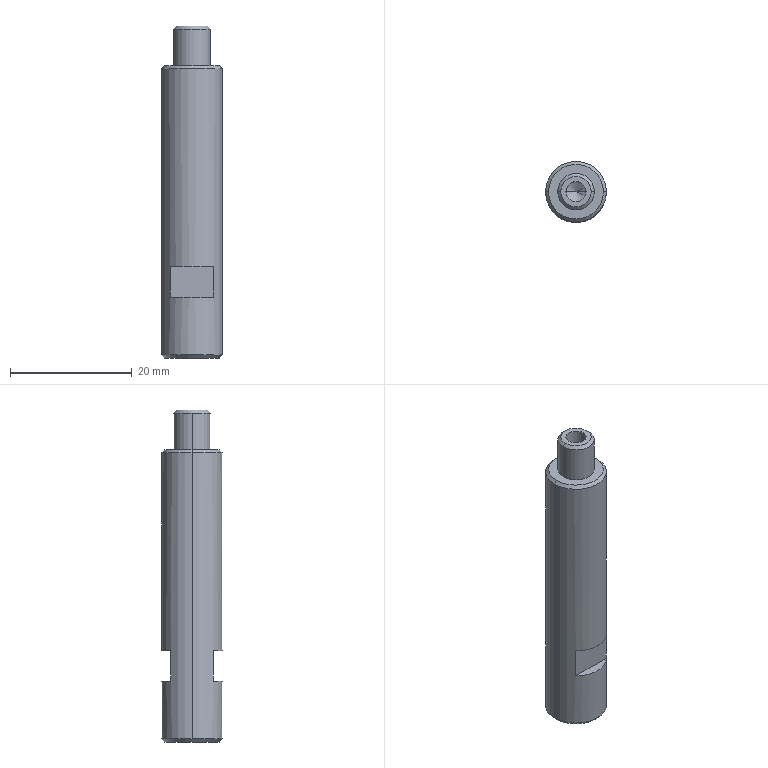Part | SolidWorks | features HoleWzd 2, ICE 2, Chamfer 1, Extrusion 1, MirrorPattern 1 | 1 solid | 27 faces | box 10 x 10 x 54.5 mm | volume 3603 mm3 | cone 10 | plane 9 | cylinder 8 | commonest cylinder face diameters 3.3 x2 4.2 x2 6 x2 10 x2
STEP:
#1=CARTESIAN_POINT('',(-4.5,0.,0.));
#2=VERTEX_POINT('',#1);
#3=CARTESIAN_POINT('',(4.5,0.,0.));
#4=VERTEX_POINT('',#3);
#5=CARTESIAN_POINT('',(0.,0.,0.));
#6=DIRECTION('',(0.,0.,-1.));
#7=DIRECTION('',(1.,0.,0.));
#8=AXIS2_PLACEMENT_3D('',#5,#6,#7);
#9=CIRCLE('',#8,4.5);
#10=EDGE_CURVE('',#2,#4,#9,.T.);
#11=ORIENTED_EDGE('',*,*,#10,.F.);
#12=CARTESIAN_POINT('',(-5.,0.,0.5));
#13=VERTEX_POINT('',#12);
#14=CARTESIAN_POINT('',(-5.,0.,0.5));
#15=DIRECTION('',(-0.7071,0.,0.7071));
#16=VECTOR('',#15,1000.);
#17=LINE('',#14,#16);
#18=EDGE_CURVE('',#2,#13,#17,.T.);
#19=ORIENTED_EDGE('',*,*,#18,.T.);
#20=CARTESIAN_POINT('',(5.,0.,0.5));
#21=VERTEX_POINT('',#20);
#22=CARTESIAN_POINT('',(0.,0.,0.5));
#23=DIRECTION('',(0.,0.,1.));
#24=DIRECTION('',(1.,0.,0.));
#25=AXIS2_PLACEMENT_3D('',#22,#23,#24);
#26=CIRCLE('',#25,5.);
#27=EDGE_CURVE('',#21,#13,#26,.T.);
#28=ORIENTED_EDGE('',*,*,#27,.F.);
#29=CARTESIAN_POINT('',(5.,0.,0.5));
#30=DIRECTION('',(0.7071,0.,0.7071));
#31=VECTOR('',#30,1000.);
#32=LINE('',#29,#31);
#33=EDGE_CURVE('',#4,#21,#32,.T.);
#34=ORIENTED_EDGE('',*,*,#33,.F.);
#35=EDGE_LOOP('',(#11,#19,#28,#34));
#36=FACE_OUTER_BOUND('',#35,.T.);
#37=CARTESIAN_POINT('',(0.,0.,0.5));
#38=DIRECTION('',(0.,0.,1.));
#39=DIRECTION('',(1.,0.,0.));
#40=AXIS2_PLACEMENT_3D('',#37,#38,#39);
#41=CONICAL_SURFACE('',#40,5.,0.7854);
#42=ADVANCED_FACE('',(#36),#41,.T.);
#43=CARTESIAN_POINT('',(4.5,0.,48.));
#44=VERTEX_POINT('',#43);
#45=CARTESIAN_POINT('',(-4.5,0.,48.));
#46=VERTEX_POINT('',#45);
#47=CARTESIAN_POINT('',(0.,0.,48.));
#48=DIRECTION('',(0.,0.,1.));
#49=DIRECTION('',(1.,0.,0.));
#50=AXIS2_PLACEMENT_3D('',#47,#48,#49);
#51=CIRCLE('',#50,4.5);
#52=EDGE_CURVE('',#44,#46,#51,.T.);
#53=ORIENTED_EDGE('',*,*,#52,.F.);
#54=CARTESIAN_POINT('',(5.,0.,47.5));
#55=VERTEX_POINT('',#54);
#56=CARTESIAN_POINT('',(4.5,0.,48.));
#57=DIRECTION('',(0.7071,0.,-0.7071));
#58=VECTOR('',#57,1000.);
#59=LINE('',#56,#58);
#60=EDGE_CURVE('',#44,#55,#59,.T.);
#61=ORIENTED_EDGE('',*,*,#60,.T.);
#62=CARTESIAN_POINT('',(-5.,0.,47.5));
#63=VERTEX_POINT('',#62);
#64=CARTESIAN_POINT('',(0.,0.,47.5));
#65=DIRECTION('',(0.,0.,-1.));
#66=DIRECTION('',(1.,0.,0.));
#67=AXIS2_PLACEMENT_3D('',#64,#65,#66);
#68=CIRCLE('',#67,5.);
#69=EDGE_CURVE('',#63,#55,#68,.T.);
#70=ORIENTED_EDGE('',*,*,#69,.F.);
#71=CARTESIAN_POINT('',(-4.5,0.,48.));
#72=DIRECTION('',(-0.7071,0.,-0.7071));
#73=VECTOR('',#72,1000.);
#74=LINE('',#71,#73);
#75=EDGE_CURVE('',#46,#63,#74,.T.);
#76=ORIENTED_EDGE('',*,*,#75,.F.);
#77=EDGE_LOOP('',(#53,#61,#70,#76));
#78=FACE_OUTER_BOUND('',#77,.T.);
#79=CARTESIAN_POINT('',(0.,0.,48.));
#80=DIRECTION('',(0.,0.,-1.));
#81=DIRECTION('',(-1.,0.,0.));
#82=AXIS2_PLACEMENT_3D('',#79,#80,#81);
#83=CONICAL_SURFACE('',#82,4.5,0.7854);
#84=ADVANCED_FACE('',(#78),#83,.T.);
#85=CARTESIAN_POINT('',(2.5,0.,54.5));
#86=VERTEX_POINT('',#85);
#87=CARTESIAN_POINT('',(-2.5,0.,54.5));
#88=VERTEX_POINT('',#87);
#89=CARTESIAN_POINT('',(0.,0.,54.5));
#90=DIRECTION('',(0.,0.,1.));
#91=DIRECTION('',(1.,0.,0.));
#92=AXIS2_PLACEMENT_3D('',#89,#90,#91);
#93=CIRCLE('',#92,2.5);
#94=EDGE_CURVE('',#86,#88,#93,.T.);
#95=ORIENTED_EDGE('',*,*,#94,.F.);
#96=CARTESIAN_POINT('',(3.,0.,54.));
#97=VERTEX_POINT('',#96);
#98=CARTESIAN_POINT('',(2.5,0.,54.5));
#99=DIRECTION('',(0.7071,0.,-0.7071));
#100=VECTOR('',#99,1000.);
#101=LINE('',#98,#100);
#102=EDGE_CURVE('',#86,#97,#101,.T.);
#103=ORIENTED_EDGE('',*,*,#102,.T.);
#104=CARTESIAN_POINT('',(-3.,0.,54.));
#105=VERTEX_POINT('',#104);
#106=CARTESIAN_POINT('',(0.,0.,54.));
#107=DIRECTION('',(0.,0.,-1.));
#108=DIRECTION('',(1.,0.,0.));
#109=AXIS2_PLACEMENT_3D('',#106,#107,#108);
#110=CIRCLE('',#109,3.);
#111=EDGE_CURVE('',#105,#97,#110,.T.);
#112=ORIENTED_EDGE('',*,*,#111,.F.);
#113=CARTESIAN_POINT('',(-2.5,0.,54.5));
#114=DIRECTION('',(-0.7071,0.,-0.7071));
#115=VECTOR('',#114,1000.);
#116=LINE('',#113,#115);
#117=EDGE_CURVE('',#88,#105,#116,.T.);
#118=ORIENTED_EDGE('',*,*,#117,.F.);
#119=EDGE_LOOP('',(#95,#103,#112,#118));
#120=FACE_OUTER_BOUND('',#119,.T.);
#121=CARTESIAN_POINT('',(0.,0.,54.5));
#122=DIRECTION('',(0.,0.,-1.));
#123=DIRECTION('',(-1.,0.,0.));
#124=AXIS2_PLACEMENT_3D('',#121,#122,#123);
#125=CONICAL_SURFACE('',#124,2.5,0.7854);
#126=ADVANCED_FACE('',(#120),#125,.T.);
#127=CARTESIAN_POINT('',(2.1,0.,12.4));
#128=VERTEX_POINT('',#127);
#129=CARTESIAN_POINT('',(-2.1,0.,12.4));
#130=VERTEX_POINT('',#129);
#131=CARTESIAN_POINT('',(0.,0.,12.4));
#132=DIRECTION('',(0.,0.,-1.));
#133=DIRECTION('',(-1.,0.,0.));
#134=AXIS2_PLACEMENT_3D('',#131,#132,#133);
#135=CIRCLE('',#134,2.1);
#136=EDGE_CURVE('',#128,#130,#135,.T.);
#137=ORIENTED_EDGE('',*,*,#136,.F.);
#138=CARTESIAN_POINT('',(2.1,0.,0.));
#139=VERTEX_POINT('',#138);
#140=CARTESIAN_POINT('',(2.1,0.,0.));
#141=DIRECTION('',(0.,0.,-1.));
#142=VECTOR('',#141,1000.);
#143=LINE('',#140,#142);
#144=EDGE_CURVE('',#128,#139,#143,.T.);
#145=ORIENTED_EDGE('',*,*,#144,.T.);
#146=CARTESIAN_POINT('',(-2.1,0.,0.));
#147=VERTEX_POINT('',#146);
#148=CARTESIAN_POINT('',(0.,0.,0.));
#149=DIRECTION('',(0.,0.,-1.));
#150=DIRECTION('',(-1.,0.,0.));
#151=AXIS2_PLACEMENT_3D('',#148,#149,#150);
#152=CIRCLE('',#151,2.1);
#153=EDGE_CURVE('',#139,#147,#152,.T.);
#154=ORIENTED_EDGE('',*,*,#153,.T.);
#155=CARTESIAN_POINT('',(-2.1,0.,0.));
#156=DIRECTION('',(0.,0.,-1.));
#157=VECTOR('',#156,1000.);
#158=LINE('',#155,#157);
#159=EDGE_CURVE('',#130,#147,#158,.T.);
#160=ORIENTED_EDGE('',*,*,#159,.F.);
#161=EDGE_LOOP('',(#137,#145,#154,#160));
#162=FACE_OUTER_BOUND('',#161,.T.);
#163=CARTESIAN_POINT('',(0.,0.,0.));
#164=DIRECTION('',(0.,0.,-1.));
#165=DIRECTION('',(-1.,0.,0.));
#166=AXIS2_PLACEMENT_3D('',#163,#164,#165);
#167=CYLINDRICAL_SURFACE('',#166,2.1);
#168=ADVANCED_FACE('',(#162),#167,.F.);
#169=CARTESIAN_POINT('',(0.,0.,13.662));
#170=VERTEX_POINT('',#169);
#171=CARTESIAN_POINT('',(-2.1,0.,12.4));
#172=DIRECTION('',(-0.8572,0.,-0.515));
#173=VECTOR('',#172,1000.);
#174=LINE('',#171,#173);
#175=EDGE_CURVE('',#170,#130,#174,.T.);
#176=ORIENTED_EDGE('',*,*,#175,.F.);
#177=CARTESIAN_POINT('',(2.1,0.,12.4));
#178=DIRECTION('',(0.8572,0.,-0.515));
#179=VECTOR('',#178,1000.);
#180=LINE('',#177,#179);
#181=EDGE_CURVE('',#170,#128,#180,.T.);
#182=ORIENTED_EDGE('',*,*,#181,.T.);
#183=ORIENTED_EDGE('',*,*,#136,.T.);
#184=EDGE_LOOP('',(#176,#182,#183));
#185=FACE_OUTER_BOUND('',#184,.T.);
#186=CARTESIAN_POINT('',(0.,0.,12.4));
#187=DIRECTION('',(0.,0.,-1.));
#188=DIRECTION('',(-1.,0.,0.));
#189=AXIS2_PLACEMENT_3D('',#186,#187,#188);
#190=CONICAL_SURFACE('',#189,2.1,1.03);
#191=ADVANCED_FACE('',(#185),#190,.F.);
#192=CARTESIAN_POINT('',(-1.65,0.,44.4));
#193=VERTEX_POINT('',#192);
#194=CARTESIAN_POINT('',(1.65,0.,44.4));
#195=VERTEX_POINT('',#194);
#196=CARTESIAN_POINT('',(0.,0.,44.4));
#197=DIRECTION('',(0.,0.,1.));
#198=DIRECTION('',(1.,0.,0.));
#199=AXIS2_PLACEMENT_3D('',#196,#197,#198);
#200=CIRCLE('',#199,1.65);
#201=EDGE_CURVE('',#193,#195,#200,.T.);
#202=ORIENTED_EDGE('',*,*,#201,.F.);
#203=CARTESIAN_POINT('',(-1.65,0.,54.5));
#204=VERTEX_POINT('',#203);
#205=CARTESIAN_POINT('',(-1.65,0.,54.5));
#206=DIRECTION('',(0.,0.,1.));
#207=VECTOR('',#206,1000.);
#208=LINE('',#205,#207);
#209=EDGE_CURVE('',#193,#204,#208,.T.);
#210=ORIENTED_EDGE('',*,*,#209,.T.);
#211=CARTESIAN_POINT('',(1.65,0.,54.5));
#212=VERTEX_POINT('',#211);
#213=CARTESIAN_POINT('',(0.,0.,54.5));
#214=DIRECTION('',(0.,0.,1.));
#215=DIRECTION('',(1.,0.,0.));
#216=AXIS2_PLACEMENT_3D('',#213,#214,#215);
#217=CIRCLE('',#216,1.65);
#218=EDGE_CURVE('',#204,#212,#217,.T.);
#219=ORIENTED_EDGE('',*,*,#218,.T.);
#220=CARTESIAN_POINT('',(1.65,0.,54.5));
#221=DIRECTION('',(0.,0.,1.));
#222=VECTOR('',#221,1000.);
#223=LINE('',#220,#222);
#224=EDGE_CURVE('',#195,#212,#223,.T.);
#225=ORIENTED_EDGE('',*,*,#224,.F.);
#226=EDGE_LOOP('',(#202,#210,#219,#225));
#227=FACE_OUTER_BOUND('',#226,.T.);
#228=CARTESIAN_POINT('',(0.,0.,54.5));
#229=DIRECTION('',(0.,0.,1.));
#230=DIRECTION('',(1.,0.,0.));
#231=AXIS2_PLACEMENT_3D('',#228,#229,#230);
#232=CYLINDRICAL_SURFACE('',#231,1.65);
#233=ADVANCED_FACE('',(#227),#232,.F.);
#234=CARTESIAN_POINT('',(0.,0.,43.409));
#235=VERTEX_POINT('',#234);
#236=CARTESIAN_POINT('',(1.65,0.,44.4));
#237=DIRECTION('',(0.8572,0.,0.515));
#238=VECTOR('',#237,1000.);
#239=LINE('',#236,#238);
#240=EDGE_CURVE('',#235,#195,#239,.T.);
#241=ORIENTED_EDGE('',*,*,#240,.F.);
#242=CARTESIAN_POINT('',(-1.65,0.,44.4));
#243=DIRECTION('',(-0.8572,0.,0.515));
#244=VECTOR('',#243,1000.);
#245=LINE('',#242,#244);
#246=EDGE_CURVE('',#235,#193,#245,.T.);
#247=ORIENTED_EDGE('',*,*,#246,.T.);
#248=ORIENTED_EDGE('',*,*,#201,.T.);
#249=EDGE_LOOP('',(#241,#247,#248));
#250=FACE_OUTER_BOUND('',#249,.T.);
#251=CARTESIAN_POINT('',(0.,0.,44.4));
#252=DIRECTION('',(0.,0.,1.));
#253=DIRECTION('',(1.,0.,0.));
#254=AXIS2_PLACEMENT_3D('',#251,#252,#253);
#255=CONICAL_SURFACE('',#254,1.65,1.03);
#256=ADVANCED_FACE('',(#250),#255,.F.);
#257=ORIENTED_EDGE('',*,*,#111,.T.);
#258=CARTESIAN_POINT('',(3.,0.,48.));
#259=VERTEX_POINT('',#258);
#260=CARTESIAN_POINT('',(3.,0.,54.5));
#261=DIRECTION('',(0.,0.,-1.));
#262=VECTOR('',#261,1000.);
#263=LINE('',#260,#262);
#264=EDGE_CURVE('',#97,#259,#263,.T.);
#265=ORIENTED_EDGE('',*,*,#264,.T.);
#266=CARTESIAN_POINT('',(-3.,0.,48.));
#267=VERTEX_POINT('',#266);
#268=CARTESIAN_POINT('',(0.,0.,48.));
#269=DIRECTION('',(0.,0.,1.));
#270=DIRECTION('',(1.,0.,0.));
#271=AXIS2_PLACEMENT_3D('',#268,#269,#270);
#272=CIRCLE('',#271,3.);
#273=EDGE_CURVE('',#259,#267,#272,.T.);
#274=ORIENTED_EDGE('',*,*,#273,.T.);
#275=CARTESIAN_POINT('',(-3.,0.,54.5));
#276=DIRECTION('',(0.,0.,-1.));
#277=VECTOR('',#276,1000.);
#278=LINE('',#275,#277);
#279=EDGE_CURVE('',#105,#267,#278,.T.);
#280=ORIENTED_EDGE('',*,*,#279,.F.);
#281=EDGE_LOOP('',(#257,#265,#274,#280));
#282=FACE_OUTER_BOUND('',#281,.T.);
#283=CARTESIAN_POINT('',(0.,0.,54.5));
#284=DIRECTION('',(0.,0.,-1.));
#285=DIRECTION('',(-1.,0.,0.));
#286=AXIS2_PLACEMENT_3D('',#283,#284,#285);
#287=CYLINDRICAL_SURFACE('',#286,3.);
#288=ADVANCED_FACE('',(#282),#287,.T.);
#289=CARTESIAN_POINT('',(3.571,3.5,15.));
#290=VERTEX_POINT('',#289);
#291=CARTESIAN_POINT('',(3.571,3.5,10.));
#292=VERTEX_POINT('',#291);
#293=CARTESIAN_POINT('',(3.571,3.5,48.));
#294=DIRECTION('',(0.,0.,-1.));
#295=VECTOR('',#294,1000.);
#296=LINE('',#293,#295);
#297=EDGE_CURVE('',#290,#292,#296,.T.);
#298=ORIENTED_EDGE('',*,*,#297,.F.);
#299=CARTESIAN_POINT('',(-3.571,3.5,15.));
#300=VERTEX_POINT('',#299);
#301=CARTESIAN_POINT('',(0.,0.,15.));
#302=DIRECTION('',(0.,0.,1.));
#303=DIRECTION('',(1.,0.,0.));
#304=AXIS2_PLACEMENT_3D('',#301,#302,#303);
#305=CIRCLE('',#304,5.);
#306=EDGE_CURVE('',#290,#300,#305,.T.);
#307=ORIENTED_EDGE('',*,*,#306,.T.);
#308=CARTESIAN_POINT('',(-3.571,3.5,10.));
#309=VERTEX_POINT('',#308);
#310=CARTESIAN_POINT('',(-3.571,3.5,48.));
#311=DIRECTION('',(0.,0.,1.));
#312=VECTOR('',#311,1000.);
#313=LINE('',#310,#312);
#314=EDGE_CURVE('',#309,#300,#313,.T.);
#315=ORIENTED_EDGE('',*,*,#314,.F.);
#316=CARTESIAN_POINT('',(0.,0.,10.));
#317=DIRECTION('',(0.,0.,-1.));
#318=DIRECTION('',(-1.,0.,0.));
#319=AXIS2_PLACEMENT_3D('',#316,#317,#318);
#320=CIRCLE('',#319,5.);
#321=EDGE_CURVE('',#309,#292,#320,.T.);
#322=ORIENTED_EDGE('',*,*,#321,.T.);
#323=EDGE_LOOP('',(#298,#307,#315,#322));
#324=FACE_BOUND('',#323,.T.);
#325=ORIENTED_EDGE('',*,*,#69,.T.);
#326=CARTESIAN_POINT('',(5.,0.,48.));
#327=DIRECTION('',(0.,0.,-1.));
#328=VECTOR('',#327,1000.);
#329=LINE('',#326,#328);
#330=EDGE_CURVE('',#55,#21,#329,.T.);
#331=ORIENTED_EDGE('',*,*,#330,.T.);
#332=ORIENTED_EDGE('',*,*,#27,.T.);
#333=CARTESIAN_POINT('',(-5.,0.,48.));
#334=DIRECTION('',(0.,0.,-1.));
#335=VECTOR('',#334,1000.);
#336=LINE('',#333,#335);
#337=EDGE_CURVE('',#63,#13,#336,.T.);
#338=ORIENTED_EDGE('',*,*,#337,.F.);
#339=EDGE_LOOP('',(#325,#331,#332,#338));
#340=FACE_OUTER_BOUND('',#339,.T.);
#341=CARTESIAN_POINT('',(0.,0.,48.));
#342=DIRECTION('',(0.,0.,-1.));
#343=DIRECTION('',(-1.,0.,0.));
#344=AXIS2_PLACEMENT_3D('',#341,#342,#343);
#345=CYLINDRICAL_SURFACE('',#344,5.);
#346=ADVANCED_FACE('',(#324,#340),#345,.T.);
#347=ORIENTED_EDGE('',*,*,#330,.F.);
#348=CARTESIAN_POINT('',(0.,0.,47.5));
#349=DIRECTION('',(0.,0.,-1.));
#350=DIRECTION('',(1.,0.,0.));
#351=AXIS2_PLACEMENT_3D('',#348,#349,#350);
#352=CIRCLE('',#351,5.);
#353=EDGE_CURVE('',#55,#63,#352,.T.);
#354=ORIENTED_EDGE('',*,*,#353,.T.);
#355=ORIENTED_EDGE('',*,*,#337,.T.);
#356=CARTESIAN_POINT('',(0.,0.,0.5));
#357=DIRECTION('',(0.,0.,1.));
#358=DIRECTION('',(1.,0.,0.));
#359=AXIS2_PLACEMENT_3D('',#356,#357,#358);
#360=CIRCLE('',#359,5.);
#361=EDGE_CURVE('',#13,#21,#360,.T.);
#362=ORIENTED_EDGE('',*,*,#361,.T.);
#363=EDGE_LOOP('',(#347,#354,#355,#362));
#364=FACE_OUTER_BOUND('',#363,.T.);
#365=CARTESIAN_POINT('',(-3.571,-3.5,15.));
#366=VERTEX_POINT('',#365);
#367=CARTESIAN_POINT('',(-3.571,-3.5,10.));
#368=VERTEX_POINT('',#367);
#369=CARTESIAN_POINT('',(-3.571,-3.5,48.));
#370=DIRECTION('',(0.,0.,-1.));
#371=VECTOR('',#370,1000.);
#372=LINE('',#369,#371);
#373=EDGE_CURVE('',#366,#368,#372,.T.);
#374=ORIENTED_EDGE('',*,*,#373,.F.);
#375=CARTESIAN_POINT('',(3.571,-3.5,15.));
#376=VERTEX_POINT('',#375);
#377=CARTESIAN_POINT('',(0.,0.,15.));
#378=DIRECTION('',(0.,0.,-1.));
#379=DIRECTION('',(-1.,0.,0.));
#380=AXIS2_PLACEMENT_3D('',#377,#378,#379);
#381=CIRCLE('',#380,5.);
#382=EDGE_CURVE('',#376,#366,#381,.T.);
#383=ORIENTED_EDGE('',*,*,#382,.F.);
#384=CARTESIAN_POINT('',(3.571,-3.5,10.));
#385=VERTEX_POINT('',#384);
#386=CARTESIAN_POINT('',(3.571,-3.5,48.));
#387=DIRECTION('',(0.,0.,1.));
#388=VECTOR('',#387,1000.);
#389=LINE('',#386,#388);
#390=EDGE_CURVE('',#385,#376,#389,.T.);
#391=ORIENTED_EDGE('',*,*,#390,.F.);
#392=CARTESIAN_POINT('',(0.,0.,10.));
#393=DIRECTION('',(0.,0.,1.));
#394=DIRECTION('',(1.,0.,0.));
#395=AXIS2_PLACEMENT_3D('',#392,#393,#394);
#396=CIRCLE('',#395,5.);
#397=EDGE_CURVE('',#368,#385,#396,.T.);
#398=ORIENTED_EDGE('',*,*,#397,.F.);
#399=EDGE_LOOP('',(#374,#383,#391,#398));
#400=FACE_BOUND('',#399,.T.);
#401=CARTESIAN_POINT('',(0.,0.,48.));
#402=DIRECTION('',(0.,0.,-1.));
#403=DIRECTION('',(-1.,0.,0.));
#404=AXIS2_PLACEMENT_3D('',#401,#402,#403);
#405=CYLINDRICAL_SURFACE('',#404,5.);
#406=ADVANCED_FACE('',(#364,#400),#405,.T.);
#407=CARTESIAN_POINT('',(0.,0.,48.));
#408=DIRECTION('',(0.,0.,1.));
#409=DIRECTION('',(1.,0.,0.));
#410=AXIS2_PLACEMENT_3D('',#407,#408,#409);
#411=CIRCLE('',#410,4.5);
#412=EDGE_CURVE('',#46,#44,#411,.T.);
#413=ORIENTED_EDGE('',*,*,#412,.T.);
#414=ORIENTED_EDGE('',*,*,#52,.T.);
#415=EDGE_LOOP('',(#413,#414));
#416=FACE_OUTER_BOUND('',#415,.T.);
#417=CARTESIAN_POINT('',(0.,0.,48.));
#418=DIRECTION('',(0.,0.,1.));
#419=DIRECTION('',(1.,0.,0.));
#420=AXIS2_PLACEMENT_3D('',#417,#418,#419);
#421=CIRCLE('',#420,3.);
#422=EDGE_CURVE('',#267,#259,#421,.T.);
#423=ORIENTED_EDGE('',*,*,#422,.F.);
#424=ORIENTED_EDGE('',*,*,#273,.F.);
#425=EDGE_LOOP('',(#423,#424));
#426=FACE_BOUND('',#425,.T.);
#427=CARTESIAN_POINT('',(0.,0.,48.));
#428=DIRECTION('',(0.,0.,1.));
#429=DIRECTION('',(1.,0.,0.));
#430=AXIS2_PLACEMENT_3D('',#427,#428,#429);
#431=PLANE('',#430);
#432=ADVANCED_FACE('',(#416,#426),#431,.T.);
#433=CARTESIAN_POINT('',(0.,0.,0.));
#434=DIRECTION('',(0.,0.,-1.));
#435=DIRECTION('',(1.,0.,0.));
#436=AXIS2_PLACEMENT_3D('',#433,#434,#435);
#437=CIRCLE('',#436,4.5);
#438=EDGE_CURVE('',#4,#2,#437,.T.);
#439=ORIENTED_EDGE('',*,*,#438,.T.);
#440=ORIENTED_EDGE('',*,*,#10,.T.);
#441=EDGE_LOOP('',(#439,#440));
#442=FACE_OUTER_BOUND('',#441,.T.);
#443=CARTESIAN_POINT('',(0.,0.,0.));
#444=DIRECTION('',(0.,0.,-1.));
#445=DIRECTION('',(-1.,0.,0.));
#446=AXIS2_PLACEMENT_3D('',#443,#444,#445);
#447=CIRCLE('',#446,2.1);
#448=EDGE_CURVE('',#147,#139,#447,.T.);
#449=ORIENTED_EDGE('',*,*,#448,.F.);
#450=ORIENTED_EDGE('',*,*,#153,.F.);
#451=EDGE_LOOP('',(#449,#450));
#452=FACE_BOUND('',#451,.T.);
#453=CARTESIAN_POINT('',(0.,0.,0.));
#454=DIRECTION('',(0.,0.,1.));
#455=DIRECTION('',(1.,0.,0.));
#456=AXIS2_PLACEMENT_3D('',#453,#454,#455);
#457=PLANE('',#456);
#458=ADVANCED_FACE('',(#442,#452),#457,.F.);
#459=ORIENTED_EDGE('',*,*,#264,.F.);
#460=CARTESIAN_POINT('',(0.,0.,54.));
#461=DIRECTION('',(0.,0.,-1.));
#462=DIRECTION('',(1.,0.,0.));
#463=AXIS2_PLACEMENT_3D('',#460,#461,#462);
#464=CIRCLE('',#463,3.);
#465=EDGE_CURVE('',#97,#105,#464,.T.);
#466=ORIENTED_EDGE('',*,*,#465,.T.);
#467=ORIENTED_EDGE('',*,*,#279,.T.);
#468=ORIENTED_EDGE('',*,*,#422,.T.);
#469=EDGE_LOOP('',(#459,#466,#467,#468));
#470=FACE_OUTER_BOUND('',#469,.T.);
#471=CARTESIAN_POINT('',(0.,0.,54.5));
#472=DIRECTION('',(0.,0.,-1.));
#473=DIRECTION('',(-1.,0.,0.));
#474=AXIS2_PLACEMENT_3D('',#471,#472,#473);
#475=CYLINDRICAL_SURFACE('',#474,3.);
#476=ADVANCED_FACE('',(#470),#475,.T.);
#477=CARTESIAN_POINT('',(0.,0.,54.5));
#478=DIRECTION('',(0.,0.,1.));
#479=DIRECTION('',(1.,0.,0.));
#480=AXIS2_PLACEMENT_3D('',#477,#478,#479);
#481=CIRCLE('',#480,2.5);
#482=EDGE_CURVE('',#88,#86,#481,.T.);
#483=ORIENTED_EDGE('',*,*,#482,.T.);
#484=ORIENTED_EDGE('',*,*,#94,.T.);
#485=EDGE_LOOP('',(#483,#484));
#486=FACE_OUTER_BOUND('',#485,.T.);
#487=CARTESIAN_POINT('',(0.,0.,54.5));
#488=DIRECTION('',(0.,0.,1.));
#489=DIRECTION('',(1.,0.,0.));
#490=AXIS2_PLACEMENT_3D('',#487,#488,#489);
#491=CIRCLE('',#490,1.65);
#492=EDGE_CURVE('',#212,#204,#491,.T.);
#493=ORIENTED_EDGE('',*,*,#492,.F.);
#494=ORIENTED_EDGE('',*,*,#218,.F.);
#495=EDGE_LOOP('',(#493,#494));
#496=FACE_BOUND('',#495,.T.);
#497=CARTESIAN_POINT('',(0.,0.,54.5));
#498=DIRECTION('',(0.,0.,1.));
#499=DIRECTION('',(1.,0.,0.));
#500=AXIS2_PLACEMENT_3D('',#497,#498,#499);
#501=PLANE('',#500);
#502=ADVANCED_FACE('',(#486,#496),#501,.T.);
#503=ORIENTED_EDGE('',*,*,#246,.F.);
#504=ORIENTED_EDGE('',*,*,#240,.T.);
#505=CARTESIAN_POINT('',(0.,0.,44.4));
#506=DIRECTION('',(0.,0.,1.));
#507=DIRECTION('',(1.,0.,0.));
#508=AXIS2_PLACEMENT_3D('',#505,#506,#507);
#509=CIRCLE('',#508,1.65);
#510=EDGE_CURVE('',#195,#193,#509,.T.);
#511=ORIENTED_EDGE('',*,*,#510,.T.);
#512=EDGE_LOOP('',(#503,#504,#511));
#513=FACE_OUTER_BOUND('',#512,.T.);
#514=CARTESIAN_POINT('',(0.,0.,44.4));
#515=DIRECTION('',(0.,0.,1.));
#516=DIRECTION('',(1.,0.,0.));
#517=AXIS2_PLACEMENT_3D('',#514,#515,#516);
#518=CONICAL_SURFACE('',#517,1.65,1.03);
#519=ADVANCED_FACE('',(#513),#518,.F.);
#520=ORIENTED_EDGE('',*,*,#209,.F.);
#521=ORIENTED_EDGE('',*,*,#510,.F.);
#522=ORIENTED_EDGE('',*,*,#224,.T.);
#523=ORIENTED_EDGE('',*,*,#492,.T.);
#524=EDGE_LOOP('',(#520,#521,#522,#523));
#525=FACE_OUTER_BOUND('',#524,.T.);
#526=CARTESIAN_POINT('',(0.,0.,54.5));
#527=DIRECTION('',(0.,0.,1.));
#528=DIRECTION('',(1.,0.,0.));
#529=AXIS2_PLACEMENT_3D('',#526,#527,#528);
#530=CYLINDRICAL_SURFACE('',#529,1.65);
#531=ADVANCED_FACE('',(#525),#530,.F.);
#532=ORIENTED_EDGE('',*,*,#181,.F.);
#533=ORIENTED_EDGE('',*,*,#175,.T.);
#534=CARTESIAN_POINT('',(0.,0.,12.4));
#535=DIRECTION('',(0.,0.,-1.));
#536=DIRECTION('',(-1.,0.,0.));
#537=AXIS2_PLACEMENT_3D('',#534,#535,#536);
#538=CIRCLE('',#537,2.1);
#539=EDGE_CURVE('',#130,#128,#538,.T.);
#540=ORIENTED_EDGE('',*,*,#539,.T.);
#541=EDGE_LOOP('',(#532,#533,#540));
#542=FACE_OUTER_BOUND('',#541,.T.);
#543=CARTESIAN_POINT('',(0.,0.,12.4));
#544=DIRECTION('',(0.,0.,-1.));
#545=DIRECTION('',(-1.,0.,0.));
#546=AXIS2_PLACEMENT_3D('',#543,#544,#545);
#547=CONICAL_SURFACE('',#546,2.1,1.03);
#548=ADVANCED_FACE('',(#542),#547,.F.);
#549=ORIENTED_EDGE('',*,*,#144,.F.);
#550=ORIENTED_EDGE('',*,*,#539,.F.);
#551=ORIENTED_EDGE('',*,*,#159,.T.);
#552=ORIENTED_EDGE('',*,*,#448,.T.);
#553=EDGE_LOOP('',(#549,#550,#551,#552));
#554=FACE_OUTER_BOUND('',#553,.T.);
#555=CARTESIAN_POINT('',(0.,0.,0.));
#556=DIRECTION('',(0.,0.,-1.));
#557=DIRECTION('',(-1.,0.,0.));
#558=AXIS2_PLACEMENT_3D('',#555,#556,#557);
#559=CYLINDRICAL_SURFACE('',#558,2.1);
#560=ADVANCED_FACE('',(#554),#559,.F.);
#561=ORIENTED_EDGE('',*,*,#102,.F.);
#562=ORIENTED_EDGE('',*,*,#482,.F.);
#563=ORIENTED_EDGE('',*,*,#117,.T.);
#564=ORIENTED_EDGE('',*,*,#465,.F.);
#565=EDGE_LOOP('',(#561,#562,#563,#564));
#566=FACE_OUTER_BOUND('',#565,.T.);
#567=CARTESIAN_POINT('',(0.,0.,54.5));
#568=DIRECTION('',(0.,0.,-1.));
#569=DIRECTION('',(-1.,0.,0.));
#570=AXIS2_PLACEMENT_3D('',#567,#568,#569);
#571=CONICAL_SURFACE('',#570,2.5,0.7854);
#572=ADVANCED_FACE('',(#566),#571,.T.);
#573=ORIENTED_EDGE('',*,*,#60,.F.);
#574=ORIENTED_EDGE('',*,*,#412,.F.);
#575=ORIENTED_EDGE('',*,*,#75,.T.);
#576=ORIENTED_EDGE('',*,*,#353,.F.);
#577=EDGE_LOOP('',(#573,#574,#575,#576));
#578=FACE_OUTER_BOUND('',#577,.T.);
#579=CARTESIAN_POINT('',(0.,0.,48.));
#580=DIRECTION('',(0.,0.,-1.));
#581=DIRECTION('',(-1.,0.,0.));
#582=AXIS2_PLACEMENT_3D('',#579,#580,#581);
#583=CONICAL_SURFACE('',#582,4.5,0.7854);
#584=ADVANCED_FACE('',(#578),#583,.T.);
#585=ORIENTED_EDGE('',*,*,#18,.F.);
#586=ORIENTED_EDGE('',*,*,#438,.F.);
#587=ORIENTED_EDGE('',*,*,#33,.T.);
#588=ORIENTED_EDGE('',*,*,#361,.F.);
#589=EDGE_LOOP('',(#585,#586,#587,#588));
#590=FACE_OUTER_BOUND('',#589,.T.);
#591=CARTESIAN_POINT('',(0.,0.,0.5));
#592=DIRECTION('',(0.,0.,1.));
#593=DIRECTION('',(1.,0.,0.));
#594=AXIS2_PLACEMENT_3D('',#591,#592,#593);
#595=CONICAL_SURFACE('',#594,5.,0.7854);
#596=ADVANCED_FACE('',(#590),#595,.T.);
#597=CARTESIAN_POINT('',(-5.,3.5,10.));
#598=DIRECTION('',(-1.,0.,0.));
#599=VECTOR('',#598,1000.);
#600=LINE('',#597,#599);
#601=EDGE_CURVE('',#292,#309,#600,.T.);
#602=ORIENTED_EDGE('',*,*,#601,.F.);
#603=ORIENTED_EDGE('',*,*,#321,.F.);
#604=EDGE_LOOP('',(#602,#603));
#605=FACE_OUTER_BOUND('',#604,.T.);
#606=CARTESIAN_POINT('',(-5.,3.5,10.));
#607=DIRECTION('',(0.,0.,-1.));
#608=DIRECTION('',(-1.,0.,0.));
#609=AXIS2_PLACEMENT_3D('',#606,#607,#608);
#610=PLANE('',#609);
#611=ADVANCED_FACE('',(#605),#610,.F.);
#612=CARTESIAN_POINT('',(-5.,3.5,15.));
#613=DIRECTION('',(1.,0.,0.));
#614=VECTOR('',#613,1000.);
#615=LINE('',#612,#614);
#616=EDGE_CURVE('',#300,#290,#615,.T.);
#617=ORIENTED_EDGE('',*,*,#616,.F.);
#618=ORIENTED_EDGE('',*,*,#306,.F.);
#619=EDGE_LOOP('',(#617,#618));
#620=FACE_OUTER_BOUND('',#619,.T.);
#621=CARTESIAN_POINT('',(-5.,3.5,15.));
#622=DIRECTION('',(0.,0.,1.));
#623=DIRECTION('',(1.,0.,0.));
#624=AXIS2_PLACEMENT_3D('',#621,#622,#623);
#625=PLANE('',#624);
#626=ADVANCED_FACE('',(#620),#625,.F.);
#627=ORIENTED_EDGE('',*,*,#297,.T.);
#628=ORIENTED_EDGE('',*,*,#601,.T.);
#629=ORIENTED_EDGE('',*,*,#314,.T.);
#630=ORIENTED_EDGE('',*,*,#616,.T.);
#631=EDGE_LOOP('',(#627,#628,#629,#630));
#632=FACE_OUTER_BOUND('',#631,.T.);
#633=CARTESIAN_POINT('',(0.,3.5,0.));
#634=DIRECTION('',(0.,1.,0.));
#635=DIRECTION('',(0.,0.,1.));
#636=AXIS2_PLACEMENT_3D('',#633,#634,#635);
#637=PLANE('',#636);
#638=ADVANCED_FACE('',(#632),#637,.T.);
#639=ORIENTED_EDGE('',*,*,#382,.T.);
#640=CARTESIAN_POINT('',(-5.,-3.5,15.));
#641=DIRECTION('',(1.,0.,0.));
#642=VECTOR('',#641,1000.);
#643=LINE('',#640,#642);
#644=EDGE_CURVE('',#366,#376,#643,.T.);
#645=ORIENTED_EDGE('',*,*,#644,.T.);
#646=EDGE_LOOP('',(#639,#645));
#647=FACE_OUTER_BOUND('',#646,.T.);
#648=CARTESIAN_POINT('',(-5.,-3.5,15.));
#649=DIRECTION('',(0.,0.,-1.));
#650=DIRECTION('',(-1.,0.,0.));
#651=AXIS2_PLACEMENT_3D('',#648,#649,#650);
#652=PLANE('',#651);
#653=ADVANCED_FACE('',(#647),#652,.T.);
#654=ORIENTED_EDGE('',*,*,#397,.T.);
#655=CARTESIAN_POINT('',(-5.,-3.5,10.));
#656=DIRECTION('',(-1.,0.,0.));
#657=VECTOR('',#656,1000.);
#658=LINE('',#655,#657);
#659=EDGE_CURVE('',#385,#368,#658,.T.);
#660=ORIENTED_EDGE('',*,*,#659,.T.);
#661=EDGE_LOOP('',(#654,#660));
#662=FACE_OUTER_BOUND('',#661,.T.);
#663=CARTESIAN_POINT('',(-5.,-3.5,10.));
#664=DIRECTION('',(0.,0.,1.));
#665=DIRECTION('',(1.,0.,0.));
#666=AXIS2_PLACEMENT_3D('',#663,#664,#665);
#667=PLANE('',#666);
#668=ADVANCED_FACE('',(#662),#667,.T.);
#669=ORIENTED_EDGE('',*,*,#373,.T.);
#670=ORIENTED_EDGE('',*,*,#659,.F.);
#671=ORIENTED_EDGE('',*,*,#390,.T.);
#672=ORIENTED_EDGE('',*,*,#644,.F.);
#673=EDGE_LOOP('',(#669,#670,#671,#672));
#674=FACE_OUTER_BOUND('',#673,.T.);
#675=CARTESIAN_POINT('',(0.,-3.5,0.));
#676=DIRECTION('',(0.,-1.,0.));
#677=DIRECTION('',(0.,0.,1.));
#678=AXIS2_PLACEMENT_3D('',#675,#676,#677);
#679=PLANE('',#678);
#680=ADVANCED_FACE('',(#674),#679,.T.);
#681=CLOSED_SHELL('',(#42,#84,#126,#168,#191,#233,#256,#288,#346,#406,#432,#458,#476,#502,#519,#531,#548,#560,#572,#584,#596,#611,#626,#638,#653,#668,#680));
#682=MANIFOLD_SOLID_BREP('',#681);
#683=CARTESIAN_POINT('',(0.,0.,0.));
#684=DIRECTION('',(0.,0.,1.));
#685=DIRECTION('',(1.,0.,0.));
#686=AXIS2_PLACEMENT_3D('',#683,#684,#685);
#687=(LENGTH_UNIT()NAMED_UNIT(*)SI_UNIT(.MILLI.,.METRE.));
#688=UNCERTAINTY_MEASURE_WITH_UNIT(LENGTH_MEASURE(0.00001),#687,'','');
#689=(NAMED_UNIT(*)PLANE_ANGLE_UNIT()SI_UNIT($,.RADIAN.));
#690=(NAMED_UNIT(*)SI_UNIT($,.STERADIAN.)SOLID_ANGLE_UNIT());
#691=(GEOMETRIC_REPRESENTATION_CONTEXT(3)GLOBAL_UNCERTAINTY_ASSIGNED_CONTEXT((#688))GLOBAL_UNIT_ASSIGNED_CONTEXT((#687,#689,#690))REPRESENTATION_CONTEXT('',''));
#692=ADVANCED_BREP_SHAPE_REPRESENTATION('',(#682,#686),#691);